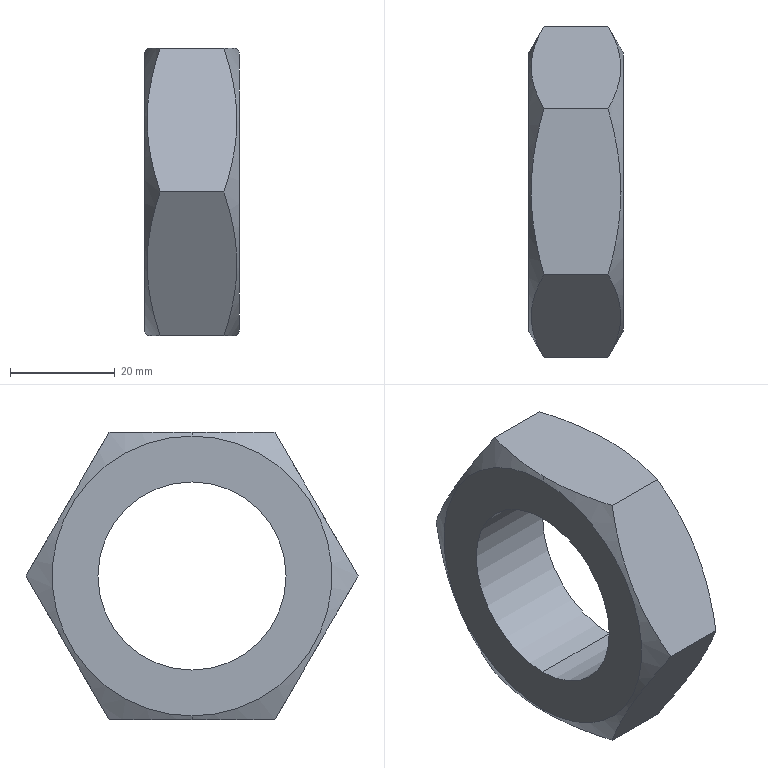Part | SolidWorks | features 3DProfileFeature 1, Extrusion 1, HoleWzd 1, MirrorPattern 1, RevCut 1 | 1 solid | 14 faces | box 18 x 63.509 x 55 mm | volume 28207 mm3 | plane 8 | cone 4 | cylinder 2 | commonest cylinder face diameters 36 x2
STEP:
#1=CARTESIAN_POINT('',(-9.,0.,26.754));
#2=VERTEX_POINT('',#1);
#3=CARTESIAN_POINT('',(-9.,0.,-26.754));
#4=VERTEX_POINT('',#3);
#5=CARTESIAN_POINT('',(-9.,0.,0.));
#6=DIRECTION('',(1.,0.,0.));
#7=DIRECTION('',(0.,0.,-1.));
#8=AXIS2_PLACEMENT_3D('',#5,#6,#7);
#9=CIRCLE('',#8,26.754);
#10=EDGE_CURVE('',#2,#4,#9,.T.);
#11=ORIENTED_EDGE('',*,*,#10,.T.);
#12=CARTESIAN_POINT('',(-8.569,0.,-27.5));
#13=VERTEX_POINT('',#12);
#14=CARTESIAN_POINT('',(-6.113,0.,-31.754));
#15=DIRECTION('',(0.5,0.,-0.866));
#16=VECTOR('',#15,1000.);
#17=LINE('',#14,#16);
#18=EDGE_CURVE('',#4,#13,#17,.T.);
#19=ORIENTED_EDGE('',*,*,#18,.T.);
#20=CARTESIAN_POINT('',(-6.113,-15.877,-27.5));
#21=VERTEX_POINT('',#20);
#22=CARTESIAN_POINT('',(-6.113,-15.877,-27.5));
#23=CARTESIAN_POINT('',(-6.486,-14.586,-27.5));
#24=CARTESIAN_POINT('',(-6.828,-13.283,-27.5));
#25=CARTESIAN_POINT('',(-7.435,-10.647,-27.5));
#26=CARTESIAN_POINT('',(-7.698,-9.325,-27.5));
#27=CARTESIAN_POINT('',(-8.339,-5.348,-27.5));
#28=CARTESIAN_POINT('',(-8.569,-2.683,-27.5));
#29=CARTESIAN_POINT('',(-8.569,0.,-27.5));
#30=B_SPLINE_CURVE_WITH_KNOTS('',3,(#22,#23,#24,#25,#26,#27,#28,#29),.UNSPECIFIED.,.F.,.F.,(4,2,2,4),(0.02826,0.03228,0.03629,0.04432),.UNSPECIFIED.);
#31=EDGE_CURVE('',#21,#13,#30,.T.);
#32=ORIENTED_EDGE('',*,*,#31,.F.);
#33=CARTESIAN_POINT('',(-6.113,-31.754,0.));
#34=VERTEX_POINT('',#33);
#35=CARTESIAN_POINT('',(-6.113,-31.754,0.));
#36=CARTESIAN_POINT('',(-6.862,-30.458,-2.245));
#37=CARTESIAN_POINT('',(-7.478,-29.152,-4.507));
#38=CARTESIAN_POINT('',(-8.333,-26.514,-9.077));
#39=CARTESIAN_POINT('',(-8.568,-25.181,-11.386));
#40=CARTESIAN_POINT('',(-8.57,-23.493,-14.308));
#41=CARTESIAN_POINT('',(-8.556,-23.154,-14.896));
#42=CARTESIAN_POINT('',(-8.499,-22.479,-16.065));
#43=CARTESIAN_POINT('',(-8.457,-22.143,-16.648));
#44=CARTESIAN_POINT('',(-8.289,-21.137,-18.391));
#45=CARTESIAN_POINT('',(-8.123,-20.47,-19.544));
#46=CARTESIAN_POINT('',(-7.481,-18.484,-22.985));
#47=CARTESIAN_POINT('',(-6.863,-17.175,-25.252));
#48=CARTESIAN_POINT('',(-6.113,-15.877,-27.5));
#49=B_SPLINE_CURVE_WITH_KNOTS('',3,(#35,#36,#37,#38,#39,#40,#41,#42,#43,#44,#45,#46,#47,#48),.UNSPECIFIED.,.F.,.F.,(4,2,2,2,2,2,4),(0.000000238,0.008018,0.01604,0.01804,0.02004,0.02405,0.03207),.UNSPECIFIED.);
#50=EDGE_CURVE('',#34,#21,#49,.T.);
#51=ORIENTED_EDGE('',*,*,#50,.F.);
#52=CARTESIAN_POINT('',(-6.113,-15.877,27.5));
#53=VERTEX_POINT('',#52);
#54=CARTESIAN_POINT('',(-6.113,-15.877,27.5));
#55=CARTESIAN_POINT('',(-6.862,-17.173,25.255));
#56=CARTESIAN_POINT('',(-7.478,-18.479,22.993));
#57=CARTESIAN_POINT('',(-8.333,-21.118,18.423));
#58=CARTESIAN_POINT('',(-8.568,-22.451,16.114));
#59=CARTESIAN_POINT('',(-8.57,-24.138,13.192));
#60=CARTESIAN_POINT('',(-8.556,-24.477,12.604));
#61=CARTESIAN_POINT('',(-8.499,-25.152,11.435));
#62=CARTESIAN_POINT('',(-8.457,-25.489,10.852));
#63=CARTESIAN_POINT('',(-8.289,-26.495,9.109));
#64=CARTESIAN_POINT('',(-8.123,-27.161,7.956));
#65=CARTESIAN_POINT('',(-7.481,-29.148,4.515));
#66=CARTESIAN_POINT('',(-6.863,-30.456,2.248));
#67=CARTESIAN_POINT('',(-6.113,-31.754,0.));
#68=B_SPLINE_CURVE_WITH_KNOTS('',3,(#54,#55,#56,#57,#58,#59,#60,#61,#62,#63,#64,#65,#66,#67),.UNSPECIFIED.,.F.,.F.,(4,2,2,2,2,2,4),(0.000000238,0.008018,0.01604,0.01804,0.02004,0.02405,0.03207),.UNSPECIFIED.);
#69=EDGE_CURVE('',#53,#34,#68,.T.);
#70=ORIENTED_EDGE('',*,*,#69,.F.);
#71=CARTESIAN_POINT('',(-8.569,0.,27.5));
#72=VERTEX_POINT('',#71);
#73=CARTESIAN_POINT('',(-8.569,0.,27.5));
#74=CARTESIAN_POINT('',(-8.569,-2.683,27.5));
#75=CARTESIAN_POINT('',(-8.339,-5.348,27.5));
#76=CARTESIAN_POINT('',(-7.698,-9.325,27.5));
#77=CARTESIAN_POINT('',(-7.435,-10.647,27.5));
#78=CARTESIAN_POINT('',(-6.828,-13.283,27.5));
#79=CARTESIAN_POINT('',(-6.486,-14.586,27.5));
#80=CARTESIAN_POINT('',(-6.113,-15.877,27.5));
#81=B_SPLINE_CURVE_WITH_KNOTS('',3,(#73,#74,#75,#76,#77,#78,#79,#80),.UNSPECIFIED.,.F.,.F.,(4,2,2,4),(0.02774,0.03575,0.03976,0.04376),.UNSPECIFIED.);
#82=EDGE_CURVE('',#72,#53,#81,.T.);
#83=ORIENTED_EDGE('',*,*,#82,.F.);
#84=CARTESIAN_POINT('',(-6.113,0.,31.754));
#85=DIRECTION('',(0.5,0.,0.866));
#86=VECTOR('',#85,1000.);
#87=LINE('',#84,#86);
#88=EDGE_CURVE('',#2,#72,#87,.T.);
#89=ORIENTED_EDGE('',*,*,#88,.F.);
#90=EDGE_LOOP('',(#11,#19,#32,#51,#70,#83,#89));
#91=FACE_OUTER_BOUND('',#90,.T.);
#92=CARTESIAN_POINT('',(-6.113,0.,0.));
#93=DIRECTION('',(1.,0.,0.));
#94=DIRECTION('',(0.,0.,1.));
#95=AXIS2_PLACEMENT_3D('',#92,#93,#94);
#96=CONICAL_SURFACE('',#95,31.754,1.047);
#97=ADVANCED_FACE('',(#91),#96,.T.);
#98=CARTESIAN_POINT('',(9.,0.,-26.754));
#99=VERTEX_POINT('',#98);
#100=CARTESIAN_POINT('',(9.,0.,26.754));
#101=VERTEX_POINT('',#100);
#102=CARTESIAN_POINT('',(9.,0.,0.));
#103=DIRECTION('',(1.,0.,0.));
#104=DIRECTION('',(0.,0.,-1.));
#105=AXIS2_PLACEMENT_3D('',#102,#103,#104);
#106=CIRCLE('',#105,26.754);
#107=EDGE_CURVE('',#99,#101,#106,.T.);
#108=ORIENTED_EDGE('',*,*,#107,.F.);
#109=CARTESIAN_POINT('',(8.569,0.,-27.5));
#110=VERTEX_POINT('',#109);
#111=CARTESIAN_POINT('',(6.113,0.,-31.754));
#112=DIRECTION('',(-0.5,0.,-0.866));
#113=VECTOR('',#112,1000.);
#114=LINE('',#111,#113);
#115=EDGE_CURVE('',#99,#110,#114,.T.);
#116=ORIENTED_EDGE('',*,*,#115,.T.);
#117=CARTESIAN_POINT('',(6.113,15.877,-27.5));
#118=VERTEX_POINT('',#117);
#119=CARTESIAN_POINT('',(6.113,15.877,-27.5));
#120=CARTESIAN_POINT('',(6.854,13.31,-27.5));
#121=CARTESIAN_POINT('',(7.472,10.709,-27.5));
#122=CARTESIAN_POINT('',(8.01,7.394,-27.5));
#123=CARTESIAN_POINT('',(8.106,6.728,-27.5));
#124=CARTESIAN_POINT('',(8.272,5.389,-27.5));
#125=CARTESIAN_POINT('',(8.342,4.715,-27.5));
#126=CARTESIAN_POINT('',(8.512,2.689,-27.5));
#127=CARTESIAN_POINT('',(8.569,1.342,-27.5));
#128=CARTESIAN_POINT('',(8.569,0.,-27.5));
#129=B_SPLINE_CURVE_WITH_KNOTS('',3,(#119,#120,#121,#122,#123,#124,#125,#126,#127,#128),.UNSPECIFIED.,.F.,.F.,(4,2,2,2,4),(0.01171,0.01972,0.02173,0.02373,0.02774),.UNSPECIFIED.);
#130=EDGE_CURVE('',#118,#110,#129,.T.);
#131=ORIENTED_EDGE('',*,*,#130,.F.);
#132=CARTESIAN_POINT('',(6.113,31.754,0.));
#133=VERTEX_POINT('',#132);
#134=CARTESIAN_POINT('',(6.113,31.754,0.));
#135=CARTESIAN_POINT('',(6.862,30.458,-2.245));
#136=CARTESIAN_POINT('',(7.478,29.152,-4.507));
#137=CARTESIAN_POINT('',(8.333,26.514,-9.077));
#138=CARTESIAN_POINT('',(8.568,25.181,-11.386));
#139=CARTESIAN_POINT('',(8.57,23.493,-14.308));
#140=CARTESIAN_POINT('',(8.556,23.154,-14.896));
#141=CARTESIAN_POINT('',(8.499,22.479,-16.065));
#142=CARTESIAN_POINT('',(8.457,22.143,-16.648));
#143=CARTESIAN_POINT('',(8.289,21.137,-18.391));
#144=CARTESIAN_POINT('',(8.123,20.47,-19.544));
#145=CARTESIAN_POINT('',(7.481,18.484,-22.985));
#146=CARTESIAN_POINT('',(6.863,17.175,-25.252));
#147=CARTESIAN_POINT('',(6.113,15.877,-27.5));
#148=B_SPLINE_CURVE_WITH_KNOTS('',3,(#134,#135,#136,#137,#138,#139,#140,#141,#142,#143,#144,#145,#146,#147),.UNSPECIFIED.,.F.,.F.,(4,2,2,2,2,2,4),(0.000000238,0.008018,0.01604,0.01804,0.02004,0.02405,0.03207),.UNSPECIFIED.);
#149=EDGE_CURVE('',#133,#118,#148,.T.);
#150=ORIENTED_EDGE('',*,*,#149,.F.);
#151=CARTESIAN_POINT('',(6.113,15.877,27.5));
#152=VERTEX_POINT('',#151);
#153=CARTESIAN_POINT('',(6.113,15.877,27.5));
#154=CARTESIAN_POINT('',(6.862,17.173,25.255));
#155=CARTESIAN_POINT('',(7.478,18.479,22.993));
#156=CARTESIAN_POINT('',(8.333,21.118,18.423));
#157=CARTESIAN_POINT('',(8.568,22.451,16.114));
#158=CARTESIAN_POINT('',(8.57,24.138,13.192));
#159=CARTESIAN_POINT('',(8.556,24.477,12.604));
#160=CARTESIAN_POINT('',(8.499,25.152,11.435));
#161=CARTESIAN_POINT('',(8.457,25.489,10.852));
#162=CARTESIAN_POINT('',(8.289,26.495,9.109));
#163=CARTESIAN_POINT('',(8.123,27.161,7.956));
#164=CARTESIAN_POINT('',(7.481,29.148,4.515));
#165=CARTESIAN_POINT('',(6.863,30.456,2.248));
#166=CARTESIAN_POINT('',(6.113,31.754,0.));
#167=B_SPLINE_CURVE_WITH_KNOTS('',3,(#153,#154,#155,#156,#157,#158,#159,#160,#161,#162,#163,#164,#165,#166),.UNSPECIFIED.,.F.,.F.,(4,2,2,2,2,2,4),(0.000000238,0.008018,0.01604,0.01804,0.02004,0.02405,0.03207),.UNSPECIFIED.);
#168=EDGE_CURVE('',#152,#133,#167,.T.);
#169=ORIENTED_EDGE('',*,*,#168,.F.);
#170=CARTESIAN_POINT('',(8.569,0.,27.5));
#171=VERTEX_POINT('',#170);
#172=CARTESIAN_POINT('',(8.569,0.,27.5));
#173=CARTESIAN_POINT('',(8.569,1.342,27.5));
#174=CARTESIAN_POINT('',(8.512,2.689,27.5));
#175=CARTESIAN_POINT('',(8.342,4.715,27.5));
#176=CARTESIAN_POINT('',(8.272,5.389,27.5));
#177=CARTESIAN_POINT('',(8.106,6.728,27.5));
#178=CARTESIAN_POINT('',(8.01,7.394,27.5));
#179=CARTESIAN_POINT('',(7.472,10.709,27.5));
#180=CARTESIAN_POINT('',(6.854,13.31,27.5));
#181=CARTESIAN_POINT('',(6.113,15.877,27.5));
#182=B_SPLINE_CURVE_WITH_KNOTS('',3,(#172,#173,#174,#175,#176,#177,#178,#179,#180,#181),.UNSPECIFIED.,.F.,.F.,(4,2,2,2,4),(0.04432,0.04834,0.05035,0.05236,0.06039),.UNSPECIFIED.);
#183=EDGE_CURVE('',#171,#152,#182,.T.);
#184=ORIENTED_EDGE('',*,*,#183,.F.);
#185=CARTESIAN_POINT('',(6.113,0.,31.754));
#186=DIRECTION('',(-0.5,0.,0.866));
#187=VECTOR('',#186,1000.);
#188=LINE('',#185,#187);
#189=EDGE_CURVE('',#101,#171,#188,.T.);
#190=ORIENTED_EDGE('',*,*,#189,.F.);
#191=EDGE_LOOP('',(#108,#116,#131,#150,#169,#184,#190));
#192=FACE_OUTER_BOUND('',#191,.T.);
#193=CARTESIAN_POINT('',(6.113,0.,0.));
#194=DIRECTION('',(-1.,0.,0.));
#195=DIRECTION('',(0.,0.,1.));
#196=AXIS2_PLACEMENT_3D('',#193,#194,#195);
#197=CONICAL_SURFACE('',#196,31.754,1.047);
#198=ADVANCED_FACE('',(#192),#197,.T.);
#199=CARTESIAN_POINT('',(9.,0.,18.));
#200=VERTEX_POINT('',#199);
#201=CARTESIAN_POINT('',(9.,0.,-18.));
#202=VERTEX_POINT('',#201);
#203=CARTESIAN_POINT('',(9.,0.,0.));
#204=DIRECTION('',(1.,0.,0.));
#205=DIRECTION('',(0.,0.,-1.));
#206=AXIS2_PLACEMENT_3D('',#203,#204,#205);
#207=CIRCLE('',#206,18.);
#208=EDGE_CURVE('',#200,#202,#207,.T.);
#209=ORIENTED_EDGE('',*,*,#208,.T.);
#210=CARTESIAN_POINT('',(-9.,0.,-18.));
#211=VERTEX_POINT('',#210);
#212=CARTESIAN_POINT('',(-9.,0.,-18.));
#213=DIRECTION('',(-1.,0.,0.));
#214=VECTOR('',#213,1000.);
#215=LINE('',#212,#214);
#216=EDGE_CURVE('',#202,#211,#215,.T.);
#217=ORIENTED_EDGE('',*,*,#216,.T.);
#218=CARTESIAN_POINT('',(-9.,0.,18.));
#219=VERTEX_POINT('',#218);
#220=CARTESIAN_POINT('',(-9.,0.,0.));
#221=DIRECTION('',(-1.,0.,0.));
#222=DIRECTION('',(0.,0.,1.));
#223=AXIS2_PLACEMENT_3D('',#220,#221,#222);
#224=CIRCLE('',#223,18.);
#225=EDGE_CURVE('',#211,#219,#224,.T.);
#226=ORIENTED_EDGE('',*,*,#225,.T.);
#227=CARTESIAN_POINT('',(-9.,0.,18.));
#228=DIRECTION('',(-1.,0.,0.));
#229=VECTOR('',#228,1000.);
#230=LINE('',#227,#229);
#231=EDGE_CURVE('',#200,#219,#230,.T.);
#232=ORIENTED_EDGE('',*,*,#231,.F.);
#233=EDGE_LOOP('',(#209,#217,#226,#232));
#234=FACE_OUTER_BOUND('',#233,.T.);
#235=CARTESIAN_POINT('',(-9.,0.,0.));
#236=DIRECTION('',(-1.,0.,0.));
#237=DIRECTION('',(0.,0.,1.));
#238=AXIS2_PLACEMENT_3D('',#235,#236,#237);
#239=CYLINDRICAL_SURFACE('',#238,18.);
#240=ADVANCED_FACE('',(#234),#239,.F.);
#241=CARTESIAN_POINT('',(6.113,-15.877,27.5));
#242=VERTEX_POINT('',#241);
#243=CARTESIAN_POINT('',(9.,-15.877,27.5));
#244=DIRECTION('',(-1.,0.,0.));
#245=VECTOR('',#244,1000.);
#246=LINE('',#243,#245);
#247=EDGE_CURVE('',#242,#53,#246,.T.);
#248=ORIENTED_EDGE('',*,*,#247,.T.);
#249=ORIENTED_EDGE('',*,*,#69,.T.);
#250=CARTESIAN_POINT('',(6.113,-31.754,0.));
#251=VERTEX_POINT('',#250);
#252=CARTESIAN_POINT('',(9.,-31.754,0.));
#253=DIRECTION('',(-1.,0.,0.));
#254=VECTOR('',#253,1000.);
#255=LINE('',#252,#254);
#256=EDGE_CURVE('',#251,#34,#255,.T.);
#257=ORIENTED_EDGE('',*,*,#256,.F.);
#258=CARTESIAN_POINT('',(6.113,-31.754,0.));
#259=CARTESIAN_POINT('',(6.862,-30.458,2.245));
#260=CARTESIAN_POINT('',(7.478,-29.152,4.507));
#261=CARTESIAN_POINT('',(8.333,-26.514,9.077));
#262=CARTESIAN_POINT('',(8.568,-25.181,11.386));
#263=CARTESIAN_POINT('',(8.57,-23.493,14.308));
#264=CARTESIAN_POINT('',(8.556,-23.154,14.896));
#265=CARTESIAN_POINT('',(8.499,-22.479,16.065));
#266=CARTESIAN_POINT('',(8.457,-22.143,16.648));
#267=CARTESIAN_POINT('',(8.289,-21.137,18.391));
#268=CARTESIAN_POINT('',(8.123,-20.47,19.544));
#269=CARTESIAN_POINT('',(7.481,-18.484,22.985));
#270=CARTESIAN_POINT('',(6.863,-17.175,25.252));
#271=CARTESIAN_POINT('',(6.113,-15.877,27.5));
#272=B_SPLINE_CURVE_WITH_KNOTS('',3,(#258,#259,#260,#261,#262,#263,#264,#265,#266,#267,#268,#269,#270,#271),.UNSPECIFIED.,.F.,.F.,(4,2,2,2,2,2,4),(0.000000238,0.008018,0.01604,0.01804,0.02004,0.02405,0.03207),.UNSPECIFIED.);
#273=EDGE_CURVE('',#251,#242,#272,.T.);
#274=ORIENTED_EDGE('',*,*,#273,.T.);
#275=EDGE_LOOP('',(#248,#249,#257,#274));
#276=FACE_OUTER_BOUND('',#275,.T.);
#277=CARTESIAN_POINT('',(9.,-15.877,27.5));
#278=DIRECTION('',(0.,0.866,-0.5));
#279=DIRECTION('',(0.,0.5,0.866));
#280=AXIS2_PLACEMENT_3D('',#277,#278,#279);
#281=PLANE('',#280);
#282=ADVANCED_FACE('',(#276),#281,.F.);
#283=ORIENTED_EDGE('',*,*,#256,.T.);
#284=ORIENTED_EDGE('',*,*,#50,.T.);
#285=CARTESIAN_POINT('',(6.113,-15.877,-27.5));
#286=VERTEX_POINT('',#285);
#287=CARTESIAN_POINT('',(9.,-15.877,-27.5));
#288=DIRECTION('',(-1.,0.,0.));
#289=VECTOR('',#288,1000.);
#290=LINE('',#287,#289);
#291=EDGE_CURVE('',#286,#21,#290,.T.);
#292=ORIENTED_EDGE('',*,*,#291,.F.);
#293=CARTESIAN_POINT('',(6.113,-15.877,-27.5));
#294=CARTESIAN_POINT('',(6.862,-17.173,-25.255));
#295=CARTESIAN_POINT('',(7.478,-18.479,-22.993));
#296=CARTESIAN_POINT('',(8.333,-21.118,-18.423));
#297=CARTESIAN_POINT('',(8.568,-22.451,-16.114));
#298=CARTESIAN_POINT('',(8.57,-24.138,-13.192));
#299=CARTESIAN_POINT('',(8.556,-24.477,-12.604));
#300=CARTESIAN_POINT('',(8.499,-25.152,-11.435));
#301=CARTESIAN_POINT('',(8.457,-25.489,-10.852));
#302=CARTESIAN_POINT('',(8.289,-26.495,-9.109));
#303=CARTESIAN_POINT('',(8.123,-27.161,-7.956));
#304=CARTESIAN_POINT('',(7.481,-29.148,-4.515));
#305=CARTESIAN_POINT('',(6.863,-30.456,-2.248));
#306=CARTESIAN_POINT('',(6.113,-31.754,0.));
#307=B_SPLINE_CURVE_WITH_KNOTS('',3,(#293,#294,#295,#296,#297,#298,#299,#300,#301,#302,#303,#304,#305,#306),.UNSPECIFIED.,.F.,.F.,(4,2,2,2,2,2,4),(0.000000238,0.008018,0.01604,0.01804,0.02004,0.02405,0.03207),.UNSPECIFIED.);
#308=EDGE_CURVE('',#286,#251,#307,.T.);
#309=ORIENTED_EDGE('',*,*,#308,.T.);
#310=EDGE_LOOP('',(#283,#284,#292,#309));
#311=FACE_OUTER_BOUND('',#310,.T.);
#312=CARTESIAN_POINT('',(9.,-31.754,0.));
#313=DIRECTION('',(0.,0.866,0.5));
#314=DIRECTION('',(0.,-0.5,0.866));
#315=AXIS2_PLACEMENT_3D('',#312,#313,#314);
#316=PLANE('',#315);
#317=ADVANCED_FACE('',(#311),#316,.F.);
#318=ORIENTED_EDGE('',*,*,#291,.T.);
#319=ORIENTED_EDGE('',*,*,#31,.T.);
#320=CARTESIAN_POINT('',(-6.113,15.877,-27.5));
#321=VERTEX_POINT('',#320);
#322=CARTESIAN_POINT('',(-8.569,0.,-27.5));
#323=CARTESIAN_POINT('',(-8.569,1.342,-27.5));
#324=CARTESIAN_POINT('',(-8.512,2.689,-27.5));
#325=CARTESIAN_POINT('',(-8.342,4.715,-27.5));
#326=CARTESIAN_POINT('',(-8.272,5.389,-27.5));
#327=CARTESIAN_POINT('',(-8.106,6.728,-27.5));
#328=CARTESIAN_POINT('',(-8.01,7.394,-27.5));
#329=CARTESIAN_POINT('',(-7.472,10.709,-27.5));
#330=CARTESIAN_POINT('',(-6.854,13.31,-27.5));
#331=CARTESIAN_POINT('',(-6.113,15.877,-27.5));
#332=B_SPLINE_CURVE_WITH_KNOTS('',3,(#322,#323,#324,#325,#326,#327,#328,#329,#330,#331),.UNSPECIFIED.,.F.,.F.,(4,2,2,2,4),(0.04432,0.04834,0.05035,0.05236,0.06039),.UNSPECIFIED.);
#333=EDGE_CURVE('',#13,#321,#332,.T.);
#334=ORIENTED_EDGE('',*,*,#333,.T.);
#335=CARTESIAN_POINT('',(9.,15.877,-27.5));
#336=DIRECTION('',(-1.,0.,0.));
#337=VECTOR('',#336,1000.);
#338=LINE('',#335,#337);
#339=EDGE_CURVE('',#118,#321,#338,.T.);
#340=ORIENTED_EDGE('',*,*,#339,.F.);
#341=ORIENTED_EDGE('',*,*,#130,.T.);
#342=CARTESIAN_POINT('',(8.569,0.,-27.5));
#343=CARTESIAN_POINT('',(8.569,-2.683,-27.5));
#344=CARTESIAN_POINT('',(8.339,-5.348,-27.5));
#345=CARTESIAN_POINT('',(7.698,-9.325,-27.5));
#346=CARTESIAN_POINT('',(7.435,-10.647,-27.5));
#347=CARTESIAN_POINT('',(6.828,-13.283,-27.5));
#348=CARTESIAN_POINT('',(6.486,-14.586,-27.5));
#349=CARTESIAN_POINT('',(6.113,-15.877,-27.5));
#350=B_SPLINE_CURVE_WITH_KNOTS('',3,(#342,#343,#344,#345,#346,#347,#348,#349),.UNSPECIFIED.,.F.,.F.,(4,2,2,4),(0.02774,0.03575,0.03976,0.04376),.UNSPECIFIED.);
#351=EDGE_CURVE('',#110,#286,#350,.T.);
#352=ORIENTED_EDGE('',*,*,#351,.T.);
#353=EDGE_LOOP('',(#318,#319,#334,#340,#341,#352));
#354=FACE_OUTER_BOUND('',#353,.T.);
#355=CARTESIAN_POINT('',(9.,-15.877,-27.5));
#356=DIRECTION('',(0.,0.,1.));
#357=DIRECTION('',(0.,-1.,0.));
#358=AXIS2_PLACEMENT_3D('',#355,#356,#357);
#359=PLANE('',#358);
#360=ADVANCED_FACE('',(#354),#359,.F.);
#361=ORIENTED_EDGE('',*,*,#339,.T.);
#362=CARTESIAN_POINT('',(-6.113,31.754,0.));
#363=VERTEX_POINT('',#362);
#364=CARTESIAN_POINT('',(-6.113,15.877,-27.5));
#365=CARTESIAN_POINT('',(-6.862,17.173,-25.255));
#366=CARTESIAN_POINT('',(-7.478,18.479,-22.993));
#367=CARTESIAN_POINT('',(-8.333,21.118,-18.423));
#368=CARTESIAN_POINT('',(-8.568,22.451,-16.114));
#369=CARTESIAN_POINT('',(-8.57,24.138,-13.192));
#370=CARTESIAN_POINT('',(-8.556,24.477,-12.604));
#371=CARTESIAN_POINT('',(-8.499,25.152,-11.435));
#372=CARTESIAN_POINT('',(-8.457,25.489,-10.852));
#373=CARTESIAN_POINT('',(-8.289,26.495,-9.109));
#374=CARTESIAN_POINT('',(-8.123,27.161,-7.956));
#375=CARTESIAN_POINT('',(-7.481,29.148,-4.515));
#376=CARTESIAN_POINT('',(-6.863,30.456,-2.248));
#377=CARTESIAN_POINT('',(-6.113,31.754,0.));
#378=B_SPLINE_CURVE_WITH_KNOTS('',3,(#364,#365,#366,#367,#368,#369,#370,#371,#372,#373,#374,#375,#376,#377),.UNSPECIFIED.,.F.,.F.,(4,2,2,2,2,2,4),(0.000000238,0.008018,0.01604,0.01804,0.02004,0.02405,0.03207),.UNSPECIFIED.);
#379=EDGE_CURVE('',#321,#363,#378,.T.);
#380=ORIENTED_EDGE('',*,*,#379,.T.);
#381=CARTESIAN_POINT('',(9.,31.754,0.));
#382=DIRECTION('',(-1.,0.,0.));
#383=VECTOR('',#382,1000.);
#384=LINE('',#381,#383);
#385=EDGE_CURVE('',#133,#363,#384,.T.);
#386=ORIENTED_EDGE('',*,*,#385,.F.);
#387=ORIENTED_EDGE('',*,*,#149,.T.);
#388=EDGE_LOOP('',(#361,#380,#386,#387));
#389=FACE_OUTER_BOUND('',#388,.T.);
#390=CARTESIAN_POINT('',(9.,15.877,-27.5));
#391=DIRECTION('',(0.,-0.866,0.5));
#392=DIRECTION('',(0.,-0.5,-0.866));
#393=AXIS2_PLACEMENT_3D('',#390,#391,#392);
#394=PLANE('',#393);
#395=ADVANCED_FACE('',(#389),#394,.F.);
#396=ORIENTED_EDGE('',*,*,#385,.T.);
#397=CARTESIAN_POINT('',(-6.113,15.877,27.5));
#398=VERTEX_POINT('',#397);
#399=CARTESIAN_POINT('',(-6.113,31.754,0.));
#400=CARTESIAN_POINT('',(-6.862,30.458,2.245));
#401=CARTESIAN_POINT('',(-7.478,29.152,4.507));
#402=CARTESIAN_POINT('',(-8.333,26.514,9.077));
#403=CARTESIAN_POINT('',(-8.568,25.181,11.386));
#404=CARTESIAN_POINT('',(-8.57,23.493,14.308));
#405=CARTESIAN_POINT('',(-8.556,23.154,14.896));
#406=CARTESIAN_POINT('',(-8.499,22.479,16.065));
#407=CARTESIAN_POINT('',(-8.457,22.143,16.648));
#408=CARTESIAN_POINT('',(-8.289,21.137,18.391));
#409=CARTESIAN_POINT('',(-8.123,20.47,19.544));
#410=CARTESIAN_POINT('',(-7.481,18.484,22.985));
#411=CARTESIAN_POINT('',(-6.863,17.175,25.252));
#412=CARTESIAN_POINT('',(-6.113,15.877,27.5));
#413=B_SPLINE_CURVE_WITH_KNOTS('',3,(#399,#400,#401,#402,#403,#404,#405,#406,#407,#408,#409,#410,#411,#412),.UNSPECIFIED.,.F.,.F.,(4,2,2,2,2,2,4),(0.000000238,0.008018,0.01604,0.01804,0.02004,0.02405,0.03207),.UNSPECIFIED.);
#414=EDGE_CURVE('',#363,#398,#413,.T.);
#415=ORIENTED_EDGE('',*,*,#414,.T.);
#416=CARTESIAN_POINT('',(9.,15.877,27.5));
#417=DIRECTION('',(-1.,0.,0.));
#418=VECTOR('',#417,1000.);
#419=LINE('',#416,#418);
#420=EDGE_CURVE('',#152,#398,#419,.T.);
#421=ORIENTED_EDGE('',*,*,#420,.F.);
#422=ORIENTED_EDGE('',*,*,#168,.T.);
#423=EDGE_LOOP('',(#396,#415,#421,#422));
#424=FACE_OUTER_BOUND('',#423,.T.);
#425=CARTESIAN_POINT('',(9.,31.754,0.));
#426=DIRECTION('',(0.,-0.866,-0.5));
#427=DIRECTION('',(0.,0.5,-0.866));
#428=AXIS2_PLACEMENT_3D('',#425,#426,#427);
#429=PLANE('',#428);
#430=ADVANCED_FACE('',(#424),#429,.F.);
#431=ORIENTED_EDGE('',*,*,#420,.T.);
#432=CARTESIAN_POINT('',(-6.113,15.877,27.5));
#433=CARTESIAN_POINT('',(-6.854,13.31,27.5));
#434=CARTESIAN_POINT('',(-7.472,10.709,27.5));
#435=CARTESIAN_POINT('',(-8.01,7.394,27.5));
#436=CARTESIAN_POINT('',(-8.106,6.728,27.5));
#437=CARTESIAN_POINT('',(-8.272,5.389,27.5));
#438=CARTESIAN_POINT('',(-8.342,4.715,27.5));
#439=CARTESIAN_POINT('',(-8.512,2.689,27.5));
#440=CARTESIAN_POINT('',(-8.569,1.342,27.5));
#441=CARTESIAN_POINT('',(-8.569,0.,27.5));
#442=B_SPLINE_CURVE_WITH_KNOTS('',3,(#432,#433,#434,#435,#436,#437,#438,#439,#440,#441),.UNSPECIFIED.,.F.,.F.,(4,2,2,2,4),(0.01171,0.01972,0.02173,0.02373,0.02774),.UNSPECIFIED.);
#443=EDGE_CURVE('',#398,#72,#442,.T.);
#444=ORIENTED_EDGE('',*,*,#443,.T.);
#445=ORIENTED_EDGE('',*,*,#82,.T.);
#446=ORIENTED_EDGE('',*,*,#247,.F.);
#447=CARTESIAN_POINT('',(6.113,-15.877,27.5));
#448=CARTESIAN_POINT('',(6.486,-14.586,27.5));
#449=CARTESIAN_POINT('',(6.828,-13.283,27.5));
#450=CARTESIAN_POINT('',(7.435,-10.647,27.5));
#451=CARTESIAN_POINT('',(7.698,-9.325,27.5));
#452=CARTESIAN_POINT('',(8.339,-5.348,27.5));
#453=CARTESIAN_POINT('',(8.569,-2.683,27.5));
#454=CARTESIAN_POINT('',(8.569,0.,27.5));
#455=B_SPLINE_CURVE_WITH_KNOTS('',3,(#447,#448,#449,#450,#451,#452,#453,#454),.UNSPECIFIED.,.F.,.F.,(4,2,2,4),(0.02826,0.03228,0.03629,0.04432),.UNSPECIFIED.);
#456=EDGE_CURVE('',#242,#171,#455,.T.);
#457=ORIENTED_EDGE('',*,*,#456,.T.);
#458=ORIENTED_EDGE('',*,*,#183,.T.);
#459=EDGE_LOOP('',(#431,#444,#445,#446,#457,#458));
#460=FACE_OUTER_BOUND('',#459,.T.);
#461=CARTESIAN_POINT('',(9.,15.877,27.5));
#462=DIRECTION('',(0.,0.,-1.));
#463=DIRECTION('',(0.,1.,0.));
#464=AXIS2_PLACEMENT_3D('',#461,#462,#463);
#465=PLANE('',#464);
#466=ADVANCED_FACE('',(#460),#465,.F.);
#467=CARTESIAN_POINT('',(9.,0.,0.));
#468=DIRECTION('',(1.,0.,0.));
#469=DIRECTION('',(0.,0.,-1.));
#470=AXIS2_PLACEMENT_3D('',#467,#468,#469);
#471=CIRCLE('',#470,26.754);
#472=EDGE_CURVE('',#101,#99,#471,.T.);
#473=ORIENTED_EDGE('',*,*,#472,.T.);
#474=ORIENTED_EDGE('',*,*,#107,.T.);
#475=EDGE_LOOP('',(#473,#474));
#476=FACE_OUTER_BOUND('',#475,.T.);
#477=ORIENTED_EDGE('',*,*,#208,.F.);
#478=CARTESIAN_POINT('',(9.,0.,0.));
#479=DIRECTION('',(1.,0.,0.));
#480=DIRECTION('',(0.,0.,-1.));
#481=AXIS2_PLACEMENT_3D('',#478,#479,#480);
#482=CIRCLE('',#481,18.);
#483=EDGE_CURVE('',#202,#200,#482,.T.);
#484=ORIENTED_EDGE('',*,*,#483,.F.);
#485=EDGE_LOOP('',(#477,#484));
#486=FACE_BOUND('',#485,.T.);
#487=CARTESIAN_POINT('',(9.,-31.754,0.));
#488=DIRECTION('',(1.,0.,0.));
#489=DIRECTION('',(0.,0.,-1.));
#490=AXIS2_PLACEMENT_3D('',#487,#488,#489);
#491=PLANE('',#490);
#492=ADVANCED_FACE('',(#476,#486),#491,.T.);
#493=ORIENTED_EDGE('',*,*,#10,.F.);
#494=CARTESIAN_POINT('',(-9.,0.,0.));
#495=DIRECTION('',(1.,0.,0.));
#496=DIRECTION('',(0.,0.,-1.));
#497=AXIS2_PLACEMENT_3D('',#494,#495,#496);
#498=CIRCLE('',#497,26.754);
#499=EDGE_CURVE('',#4,#2,#498,.T.);
#500=ORIENTED_EDGE('',*,*,#499,.F.);
#501=EDGE_LOOP('',(#493,#500));
#502=FACE_OUTER_BOUND('',#501,.T.);
#503=CARTESIAN_POINT('',(-9.,0.,0.));
#504=DIRECTION('',(-1.,0.,0.));
#505=DIRECTION('',(0.,0.,1.));
#506=AXIS2_PLACEMENT_3D('',#503,#504,#505);
#507=CIRCLE('',#506,18.);
#508=EDGE_CURVE('',#219,#211,#507,.T.);
#509=ORIENTED_EDGE('',*,*,#508,.F.);
#510=ORIENTED_EDGE('',*,*,#225,.F.);
#511=EDGE_LOOP('',(#509,#510));
#512=FACE_BOUND('',#511,.T.);
#513=CARTESIAN_POINT('',(-9.,-31.754,0.));
#514=DIRECTION('',(1.,0.,0.));
#515=DIRECTION('',(0.,0.,-1.));
#516=AXIS2_PLACEMENT_3D('',#513,#514,#515);
#517=PLANE('',#516);
#518=ADVANCED_FACE('',(#502,#512),#517,.F.);
#519=ORIENTED_EDGE('',*,*,#216,.F.);
#520=ORIENTED_EDGE('',*,*,#483,.T.);
#521=ORIENTED_EDGE('',*,*,#231,.T.);
#522=ORIENTED_EDGE('',*,*,#508,.T.);
#523=EDGE_LOOP('',(#519,#520,#521,#522));
#524=FACE_OUTER_BOUND('',#523,.T.);
#525=CARTESIAN_POINT('',(-9.,0.,0.));
#526=DIRECTION('',(-1.,0.,0.));
#527=DIRECTION('',(0.,0.,1.));
#528=AXIS2_PLACEMENT_3D('',#525,#526,#527);
#529=CYLINDRICAL_SURFACE('',#528,18.);
#530=ADVANCED_FACE('',(#524),#529,.F.);
#531=ORIENTED_EDGE('',*,*,#115,.F.);
#532=ORIENTED_EDGE('',*,*,#472,.F.);
#533=ORIENTED_EDGE('',*,*,#189,.T.);
#534=ORIENTED_EDGE('',*,*,#456,.F.);
#535=ORIENTED_EDGE('',*,*,#273,.F.);
#536=ORIENTED_EDGE('',*,*,#308,.F.);
#537=ORIENTED_EDGE('',*,*,#351,.F.);
#538=EDGE_LOOP('',(#531,#532,#533,#534,#535,#536,#537));
#539=FACE_OUTER_BOUND('',#538,.T.);
#540=CARTESIAN_POINT('',(6.113,0.,0.));
#541=DIRECTION('',(-1.,0.,0.));
#542=DIRECTION('',(0.,0.,1.));
#543=AXIS2_PLACEMENT_3D('',#540,#541,#542);
#544=CONICAL_SURFACE('',#543,31.754,1.047);
#545=ADVANCED_FACE('',(#539),#544,.T.);
#546=ORIENTED_EDGE('',*,*,#18,.F.);
#547=ORIENTED_EDGE('',*,*,#499,.T.);
#548=ORIENTED_EDGE('',*,*,#88,.T.);
#549=ORIENTED_EDGE('',*,*,#443,.F.);
#550=ORIENTED_EDGE('',*,*,#414,.F.);
#551=ORIENTED_EDGE('',*,*,#379,.F.);
#552=ORIENTED_EDGE('',*,*,#333,.F.);
#553=EDGE_LOOP('',(#546,#547,#548,#549,#550,#551,#552));
#554=FACE_OUTER_BOUND('',#553,.T.);
#555=CARTESIAN_POINT('',(-6.113,0.,0.));
#556=DIRECTION('',(1.,0.,0.));
#557=DIRECTION('',(0.,0.,1.));
#558=AXIS2_PLACEMENT_3D('',#555,#556,#557);
#559=CONICAL_SURFACE('',#558,31.754,1.047);
#560=ADVANCED_FACE('',(#554),#559,.T.);
#561=CLOSED_SHELL('',(#97,#198,#240,#282,#317,#360,#395,#430,#466,#492,#518,#530,#545,#560));
#562=MANIFOLD_SOLID_BREP('',#561);
#563=CARTESIAN_POINT('',(0.,0.,0.));
#564=DIRECTION('',(0.,0.,1.));
#565=DIRECTION('',(1.,0.,0.));
#566=AXIS2_PLACEMENT_3D('',#563,#564,#565);
#567=(LENGTH_UNIT()NAMED_UNIT(*)SI_UNIT(.MILLI.,.METRE.));
#568=UNCERTAINTY_MEASURE_WITH_UNIT(LENGTH_MEASURE(0.00001),#567,'','');
#569=(NAMED_UNIT(*)PLANE_ANGLE_UNIT()SI_UNIT($,.RADIAN.));
#570=(NAMED_UNIT(*)SI_UNIT($,.STERADIAN.)SOLID_ANGLE_UNIT());
#571=(GEOMETRIC_REPRESENTATION_CONTEXT(3)GLOBAL_UNCERTAINTY_ASSIGNED_CONTEXT((#568))GLOBAL_UNIT_ASSIGNED_CONTEXT((#567,#569,#570))REPRESENTATION_CONTEXT('',''));
#572=ADVANCED_BREP_SHAPE_REPRESENTATION('',(#562,#566),#571);